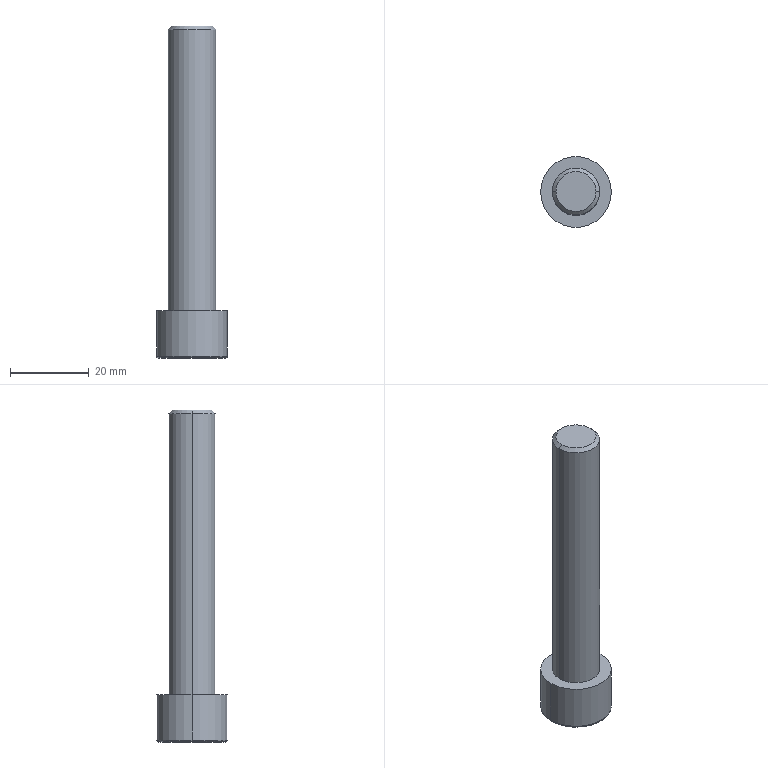Part | Creo | 1 solid | 20 faces | box 18 x 18 x 84.5 mm | volume 10550 mm3 | plane 10 | torus 4 | cylinder 4 | cone 2 | commonest cylinder face diameters 12 x2 18 x2
STEP:
#1=CARTESIAN_POINT('',(56.5,-5.,-119.5));
#2=VERTEX_POINT('',#1);
#3=CARTESIAN_POINT('',(73.5,-5.,-119.5));
#4=VERTEX_POINT('',#3);
#5=CARTESIAN_POINT('',(65.,-5.,-119.5));
#6=DIRECTION('',(0.,0.,-1.));
#7=DIRECTION('',(-1.,0.,0.));
#8=AXIS2_PLACEMENT_3D('',#5,#6,#7);
#9=CIRCLE('',#8,8.5);
#10=EDGE_CURVE('',#2,#4,#9,.T.);
#11=ORIENTED_EDGE('',*,*,#10,.F.);
#12=CARTESIAN_POINT('',(65.,-5.,-119.5));
#13=DIRECTION('',(0.,0.,-1.));
#14=DIRECTION('',(1.,0.,0.));
#15=AXIS2_PLACEMENT_3D('',#12,#13,#14);
#16=CIRCLE('',#15,8.5);
#17=EDGE_CURVE('',#4,#2,#16,.T.);
#18=ORIENTED_EDGE('',*,*,#17,.F.);
#19=EDGE_LOOP('',(#11,#18));
#20=FACE_OUTER_BOUND('',#19,.F.);
#21=CARTESIAN_POINT('',(62.113,0.,-119.5));
#22=VERTEX_POINT('',#21);
#23=CARTESIAN_POINT('',(67.887,0.,-119.5));
#24=VERTEX_POINT('',#23);
#25=CARTESIAN_POINT('',(62.113,0.,-119.5));
#26=DIRECTION('',(1.,0.,0.));
#27=VECTOR('',#26,5.774);
#28=LINE('',#25,#27);
#29=EDGE_CURVE('',#22,#24,#28,.T.);
#30=ORIENTED_EDGE('',*,*,#29,.T.);
#31=CARTESIAN_POINT('',(70.774,-5.,-119.5));
#32=VERTEX_POINT('',#31);
#33=CARTESIAN_POINT('',(70.774,-5.,-119.5));
#34=DIRECTION('',(-0.5,0.866,0.));
#35=VECTOR('',#34,5.774);
#36=LINE('',#33,#35);
#37=EDGE_CURVE('',#32,#24,#36,.T.);
#38=ORIENTED_EDGE('',*,*,#37,.F.);
#39=CARTESIAN_POINT('',(67.887,-10.,-119.5));
#40=VERTEX_POINT('',#39);
#41=CARTESIAN_POINT('',(67.887,-10.,-119.5));
#42=DIRECTION('',(0.5,0.866,0.));
#43=VECTOR('',#42,5.774);
#44=LINE('',#41,#43);
#45=EDGE_CURVE('',#40,#32,#44,.T.);
#46=ORIENTED_EDGE('',*,*,#45,.F.);
#47=CARTESIAN_POINT('',(62.113,-10.,-119.5));
#48=VERTEX_POINT('',#47);
#49=CARTESIAN_POINT('',(67.887,-10.,-119.5));
#50=DIRECTION('',(-1.,0.,0.));
#51=VECTOR('',#50,5.774);
#52=LINE('',#49,#51);
#53=EDGE_CURVE('',#40,#48,#52,.T.);
#54=ORIENTED_EDGE('',*,*,#53,.T.);
#55=CARTESIAN_POINT('',(59.226,-5.,-119.5));
#56=VERTEX_POINT('',#55);
#57=CARTESIAN_POINT('',(59.226,-5.,-119.5));
#58=DIRECTION('',(0.5,-0.866,0.));
#59=VECTOR('',#58,5.774);
#60=LINE('',#57,#59);
#61=EDGE_CURVE('',#56,#48,#60,.T.);
#62=ORIENTED_EDGE('',*,*,#61,.F.);
#63=CARTESIAN_POINT('',(62.113,0.,-119.5));
#64=DIRECTION('',(-0.5,-0.866,0.));
#65=VECTOR('',#64,5.774);
#66=LINE('',#63,#65);
#67=EDGE_CURVE('',#22,#56,#66,.T.);
#68=ORIENTED_EDGE('',*,*,#67,.F.);
#69=EDGE_LOOP('',(#30,#38,#46,#54,#62,#68));
#70=FACE_BOUND('',#69,.F.);
#71=CARTESIAN_POINT('',(65.,-5.,-119.5));
#72=DIRECTION('',(0.,0.,-1.));
#73=DIRECTION('',(-1.,0.,0.));
#74=AXIS2_PLACEMENT_3D('',#71,#72,#73);
#75=PLANE('',#74);
#76=ADVANCED_FACE('',(#20,#70),#75,.T.);
#77=ORIENTED_EDGE('',*,*,#10,.T.);
#78=CARTESIAN_POINT('',(73.854,-5.,-119.354));
#79=VERTEX_POINT('',#78);
#80=CARTESIAN_POINT('',(73.5,-5.,-119.));
#81=DIRECTION('',(0.,1.,0.));
#82=DIRECTION('',(0.7071,0.,-0.7071));
#83=AXIS2_PLACEMENT_3D('',#80,#81,#82);
#84=CIRCLE('',#83,0.5);
#85=EDGE_CURVE('',#79,#4,#84,.T.);
#86=ORIENTED_EDGE('',*,*,#85,.F.);
#87=CARTESIAN_POINT('',(56.146,-5.,-119.354));
#88=VERTEX_POINT('',#87);
#89=CARTESIAN_POINT('',(65.,-5.,-119.354));
#90=DIRECTION('',(0.,0.,-1.));
#91=DIRECTION('',(-1.,0.,0.));
#92=AXIS2_PLACEMENT_3D('',#89,#90,#91);
#93=CIRCLE('',#92,8.854);
#94=EDGE_CURVE('',#88,#79,#93,.T.);
#95=ORIENTED_EDGE('',*,*,#94,.F.);
#96=CARTESIAN_POINT('',(56.5,-5.,-119.));
#97=DIRECTION('',(0.,-1.,0.));
#98=DIRECTION('',(-0.7071,0.,-0.7071));
#99=AXIS2_PLACEMENT_3D('',#96,#97,#98);
#100=CIRCLE('',#99,0.5);
#101=EDGE_CURVE('',#88,#2,#100,.T.);
#102=ORIENTED_EDGE('',*,*,#101,.T.);
#103=EDGE_LOOP('',(#77,#86,#95,#102));
#104=FACE_OUTER_BOUND('',#103,.F.);
#105=CARTESIAN_POINT('',(65.,-5.,-119.));
#106=DIRECTION('',(0.,0.,-1.));
#107=DIRECTION('',(-1.,0.,0.));
#108=AXIS2_PLACEMENT_3D('',#105,#106,#107);
#109=TOROIDAL_SURFACE('',#108,8.5,0.5);
#110=ADVANCED_FACE('',(#104),#109,.T.);
#111=ORIENTED_EDGE('',*,*,#17,.T.);
#112=ORIENTED_EDGE('',*,*,#101,.F.);
#113=CARTESIAN_POINT('',(65.,-5.,-119.354));
#114=DIRECTION('',(0.,0.,-1.));
#115=DIRECTION('',(1.,0.,0.));
#116=AXIS2_PLACEMENT_3D('',#113,#114,#115);
#117=CIRCLE('',#116,8.854);
#118=EDGE_CURVE('',#79,#88,#117,.T.);
#119=ORIENTED_EDGE('',*,*,#118,.F.);
#120=ORIENTED_EDGE('',*,*,#85,.T.);
#121=EDGE_LOOP('',(#111,#112,#119,#120));
#122=FACE_OUTER_BOUND('',#121,.F.);
#123=CARTESIAN_POINT('',(65.,-5.,-119.));
#124=DIRECTION('',(0.,0.,-1.));
#125=DIRECTION('',(-1.,0.,0.));
#126=AXIS2_PLACEMENT_3D('',#123,#124,#125);
#127=TOROIDAL_SURFACE('',#126,8.5,0.5);
#128=ADVANCED_FACE('',(#122),#127,.T.);
#129=CARTESIAN_POINT('',(74.,-5.,-119.));
#130=VERTEX_POINT('',#129);
#131=CARTESIAN_POINT('',(56.,-5.,-119.));
#132=VERTEX_POINT('',#131);
#133=CARTESIAN_POINT('',(65.,-5.,-119.));
#134=DIRECTION('',(0.,0.,-1.));
#135=DIRECTION('',(1.,0.,0.));
#136=AXIS2_PLACEMENT_3D('',#133,#134,#135);
#137=CIRCLE('',#136,9.);
#138=EDGE_CURVE('',#130,#132,#137,.T.);
#139=ORIENTED_EDGE('',*,*,#138,.F.);
#140=CARTESIAN_POINT('',(73.5,-5.,-119.));
#141=DIRECTION('',(0.,1.,0.));
#142=DIRECTION('',(1.,0.,0.));
#143=AXIS2_PLACEMENT_3D('',#140,#141,#142);
#144=CIRCLE('',#143,0.5);
#145=EDGE_CURVE('',#130,#79,#144,.T.);
#146=ORIENTED_EDGE('',*,*,#145,.T.);
#147=ORIENTED_EDGE('',*,*,#118,.T.);
#148=CARTESIAN_POINT('',(56.5,-5.,-119.));
#149=DIRECTION('',(0.,-1.,0.));
#150=DIRECTION('',(-1.,0.,0.));
#151=AXIS2_PLACEMENT_3D('',#148,#149,#150);
#152=CIRCLE('',#151,0.5);
#153=EDGE_CURVE('',#132,#88,#152,.T.);
#154=ORIENTED_EDGE('',*,*,#153,.F.);
#155=EDGE_LOOP('',(#139,#146,#147,#154));
#156=FACE_OUTER_BOUND('',#155,.F.);
#157=CARTESIAN_POINT('',(65.,-5.,-119.));
#158=DIRECTION('',(0.,0.,-1.));
#159=DIRECTION('',(-1.,0.,0.));
#160=AXIS2_PLACEMENT_3D('',#157,#158,#159);
#161=TOROIDAL_SURFACE('',#160,8.5,0.5);
#162=ADVANCED_FACE('',(#156),#161,.T.);
#163=ORIENTED_EDGE('',*,*,#138,.T.);
#164=CARTESIAN_POINT('',(56.,-5.,-107.5));
#165=VERTEX_POINT('',#164);
#166=CARTESIAN_POINT('',(56.,-5.,-107.5));
#167=DIRECTION('',(0.,0.,-1.));
#168=VECTOR('',#167,11.5);
#169=LINE('',#166,#168);
#170=EDGE_CURVE('',#165,#132,#169,.T.);
#171=ORIENTED_EDGE('',*,*,#170,.F.);
#172=CARTESIAN_POINT('',(74.,-5.,-107.5));
#173=VERTEX_POINT('',#172);
#174=CARTESIAN_POINT('',(65.,-5.,-107.5));
#175=DIRECTION('',(0.,0.,1.));
#176=DIRECTION('',(-1.,0.,0.));
#177=AXIS2_PLACEMENT_3D('',#174,#175,#176);
#178=CIRCLE('',#177,9.);
#179=EDGE_CURVE('',#165,#173,#178,.T.);
#180=ORIENTED_EDGE('',*,*,#179,.T.);
#181=CARTESIAN_POINT('',(74.,-5.,-107.5));
#182=DIRECTION('',(0.,0.,-1.));
#183=VECTOR('',#182,11.5);
#184=LINE('',#181,#183);
#185=EDGE_CURVE('',#173,#130,#184,.T.);
#186=ORIENTED_EDGE('',*,*,#185,.T.);
#187=EDGE_LOOP('',(#163,#171,#180,#186));
#188=FACE_OUTER_BOUND('',#187,.F.);
#189=CARTESIAN_POINT('',(65.,-5.,-107.5));
#190=DIRECTION('',(0.,0.,-1.));
#191=DIRECTION('',(-1.,0.,0.));
#192=AXIS2_PLACEMENT_3D('',#189,#190,#191);
#193=CYLINDRICAL_SURFACE('',#192,9.);
#194=ADVANCED_FACE('',(#188),#193,.T.);
#195=CARTESIAN_POINT('',(65.,-5.,-119.));
#196=DIRECTION('',(0.,0.,-1.));
#197=DIRECTION('',(-1.,0.,0.));
#198=AXIS2_PLACEMENT_3D('',#195,#196,#197);
#199=CIRCLE('',#198,9.);
#200=EDGE_CURVE('',#132,#130,#199,.T.);
#201=ORIENTED_EDGE('',*,*,#200,.T.);
#202=ORIENTED_EDGE('',*,*,#185,.F.);
#203=CARTESIAN_POINT('',(65.,-5.,-107.5));
#204=DIRECTION('',(0.,0.,1.));
#205=DIRECTION('',(1.,0.,0.));
#206=AXIS2_PLACEMENT_3D('',#203,#204,#205);
#207=CIRCLE('',#206,9.);
#208=EDGE_CURVE('',#173,#165,#207,.T.);
#209=ORIENTED_EDGE('',*,*,#208,.T.);
#210=ORIENTED_EDGE('',*,*,#170,.T.);
#211=EDGE_LOOP('',(#201,#202,#209,#210));
#212=FACE_OUTER_BOUND('',#211,.F.);
#213=CARTESIAN_POINT('',(65.,-5.,-107.5));
#214=DIRECTION('',(0.,0.,-1.));
#215=DIRECTION('',(-1.,0.,0.));
#216=AXIS2_PLACEMENT_3D('',#213,#214,#215);
#217=CYLINDRICAL_SURFACE('',#216,9.);
#218=ADVANCED_FACE('',(#212),#217,.T.);
#219=ORIENTED_EDGE('',*,*,#200,.F.);
#220=ORIENTED_EDGE('',*,*,#153,.T.);
#221=ORIENTED_EDGE('',*,*,#94,.T.);
#222=ORIENTED_EDGE('',*,*,#145,.F.);
#223=EDGE_LOOP('',(#219,#220,#221,#222));
#224=FACE_OUTER_BOUND('',#223,.F.);
#225=CARTESIAN_POINT('',(65.,-5.,-119.));
#226=DIRECTION('',(0.,0.,-1.));
#227=DIRECTION('',(-1.,0.,0.));
#228=AXIS2_PLACEMENT_3D('',#225,#226,#227);
#229=TOROIDAL_SURFACE('',#228,8.5,0.5);
#230=ADVANCED_FACE('',(#224),#229,.T.);
#231=ORIENTED_EDGE('',*,*,#179,.F.);
#232=ORIENTED_EDGE('',*,*,#208,.F.);
#233=EDGE_LOOP('',(#231,#232));
#234=FACE_OUTER_BOUND('',#233,.F.);
#235=CARTESIAN_POINT('',(59.,-5.,-107.5));
#236=VERTEX_POINT('',#235);
#237=CARTESIAN_POINT('',(71.,-5.,-107.5));
#238=VERTEX_POINT('',#237);
#239=CARTESIAN_POINT('',(65.,-5.,-107.5));
#240=DIRECTION('',(0.,0.,-1.));
#241=DIRECTION('',(-1.,0.,0.));
#242=AXIS2_PLACEMENT_3D('',#239,#240,#241);
#243=CIRCLE('',#242,6.);
#244=EDGE_CURVE('',#236,#238,#243,.T.);
#245=ORIENTED_EDGE('',*,*,#244,.F.);
#246=CARTESIAN_POINT('',(65.,-5.,-107.5));
#247=DIRECTION('',(0.,0.,-1.));
#248=DIRECTION('',(1.,0.,0.));
#249=AXIS2_PLACEMENT_3D('',#246,#247,#248);
#250=CIRCLE('',#249,6.);
#251=EDGE_CURVE('',#238,#236,#250,.T.);
#252=ORIENTED_EDGE('',*,*,#251,.F.);
#253=EDGE_LOOP('',(#245,#252));
#254=FACE_BOUND('',#253,.F.);
#255=CARTESIAN_POINT('',(65.,-5.,-107.5));
#256=DIRECTION('',(0.,0.,1.));
#257=DIRECTION('',(1.,0.,0.));
#258=AXIS2_PLACEMENT_3D('',#255,#256,#257);
#259=PLANE('',#258);
#260=ADVANCED_FACE('',(#234,#254),#259,.T.);
#261=CARTESIAN_POINT('',(71.,-5.,-35.9));
#262=VERTEX_POINT('',#261);
#263=CARTESIAN_POINT('',(59.,-5.,-35.9));
#264=VERTEX_POINT('',#263);
#265=CARTESIAN_POINT('',(65.,-5.,-35.9));
#266=DIRECTION('',(0.,0.,1.));
#267=DIRECTION('',(1.,0.,0.));
#268=AXIS2_PLACEMENT_3D('',#265,#266,#267);
#269=CIRCLE('',#268,6.);
#270=EDGE_CURVE('',#262,#264,#269,.T.);
#271=ORIENTED_EDGE('',*,*,#270,.T.);
#272=CARTESIAN_POINT('',(59.,-5.,-35.9));
#273=DIRECTION('',(0.,0.,-1.));
#274=VECTOR('',#273,71.6);
#275=LINE('',#272,#274);
#276=EDGE_CURVE('',#264,#236,#275,.T.);
#277=ORIENTED_EDGE('',*,*,#276,.T.);
#278=ORIENTED_EDGE('',*,*,#244,.T.);
#279=CARTESIAN_POINT('',(71.,-5.,-35.9));
#280=DIRECTION('',(0.,0.,-1.));
#281=VECTOR('',#280,71.6);
#282=LINE('',#279,#281);
#283=EDGE_CURVE('',#262,#238,#282,.T.);
#284=ORIENTED_EDGE('',*,*,#283,.F.);
#285=EDGE_LOOP('',(#271,#277,#278,#284));
#286=FACE_OUTER_BOUND('',#285,.F.);
#287=CARTESIAN_POINT('',(65.,-5.,-37.5));
#288=DIRECTION('',(0.,0.,-1.));
#289=DIRECTION('',(-1.,0.,0.));
#290=AXIS2_PLACEMENT_3D('',#287,#288,#289);
#291=CYLINDRICAL_SURFACE('',#290,6.);
#292=ADVANCED_FACE('',(#286),#291,.T.);
#293=CARTESIAN_POINT('',(70.1,-5.,-35.));
#294=VERTEX_POINT('',#293);
#295=CARTESIAN_POINT('',(59.9,-5.,-35.));
#296=VERTEX_POINT('',#295);
#297=CARTESIAN_POINT('',(65.,-5.,-35.));
#298=DIRECTION('',(0.,0.,1.));
#299=DIRECTION('',(1.,0.,0.));
#300=AXIS2_PLACEMENT_3D('',#297,#298,#299);
#301=CIRCLE('',#300,5.1);
#302=EDGE_CURVE('',#294,#296,#301,.T.);
#303=ORIENTED_EDGE('',*,*,#302,.T.);
#304=CARTESIAN_POINT('',(59.9,-5.,-35.));
#305=DIRECTION('',(-0.7071,0.,-0.7071));
#306=VECTOR('',#305,1.273);
#307=LINE('',#304,#306);
#308=EDGE_CURVE('',#296,#264,#307,.T.);
#309=ORIENTED_EDGE('',*,*,#308,.T.);
#310=ORIENTED_EDGE('',*,*,#270,.F.);
#311=CARTESIAN_POINT('',(70.1,-5.,-35.));
#312=DIRECTION('',(0.7071,0.,-0.7071));
#313=VECTOR('',#312,1.273);
#314=LINE('',#311,#313);
#315=EDGE_CURVE('',#294,#262,#314,.T.);
#316=ORIENTED_EDGE('',*,*,#315,.F.);
#317=EDGE_LOOP('',(#303,#309,#310,#316));
#318=FACE_OUTER_BOUND('',#317,.F.);
#319=CARTESIAN_POINT('',(65.,-5.,-35.45));
#320=DIRECTION('',(0.,0.,-1.));
#321=DIRECTION('',(-1.,0.,0.));
#322=AXIS2_PLACEMENT_3D('',#319,#320,#321);
#323=CONICAL_SURFACE('',#322,5.55,45.);
#324=ADVANCED_FACE('',(#318),#323,.T.);
#325=CARTESIAN_POINT('',(65.,-5.,-35.));
#326=DIRECTION('',(0.,0.,1.));
#327=DIRECTION('',(-1.,0.,0.));
#328=AXIS2_PLACEMENT_3D('',#325,#326,#327);
#329=CIRCLE('',#328,5.1);
#330=EDGE_CURVE('',#296,#294,#329,.T.);
#331=ORIENTED_EDGE('',*,*,#330,.F.);
#332=ORIENTED_EDGE('',*,*,#302,.F.);
#333=EDGE_LOOP('',(#331,#332));
#334=FACE_OUTER_BOUND('',#333,.F.);
#335=CARTESIAN_POINT('',(65.,-5.,-35.));
#336=DIRECTION('',(0.,0.,-1.));
#337=DIRECTION('',(-1.,0.,0.));
#338=AXIS2_PLACEMENT_3D('',#335,#336,#337);
#339=PLANE('',#338);
#340=ADVANCED_FACE('',(#334),#339,.F.);
#341=ORIENTED_EDGE('',*,*,#330,.T.);
#342=ORIENTED_EDGE('',*,*,#315,.T.);
#343=CARTESIAN_POINT('',(65.,-5.,-35.9));
#344=DIRECTION('',(0.,0.,1.));
#345=DIRECTION('',(-1.,0.,0.));
#346=AXIS2_PLACEMENT_3D('',#343,#344,#345);
#347=CIRCLE('',#346,6.);
#348=EDGE_CURVE('',#264,#262,#347,.T.);
#349=ORIENTED_EDGE('',*,*,#348,.F.);
#350=ORIENTED_EDGE('',*,*,#308,.F.);
#351=EDGE_LOOP('',(#341,#342,#349,#350));
#352=FACE_OUTER_BOUND('',#351,.F.);
#353=CARTESIAN_POINT('',(65.,-5.,-35.45));
#354=DIRECTION('',(0.,0.,-1.));
#355=DIRECTION('',(-1.,0.,0.));
#356=AXIS2_PLACEMENT_3D('',#353,#354,#355);
#357=CONICAL_SURFACE('',#356,5.55,45.);
#358=ADVANCED_FACE('',(#352),#357,.T.);
#359=ORIENTED_EDGE('',*,*,#348,.T.);
#360=ORIENTED_EDGE('',*,*,#283,.T.);
#361=ORIENTED_EDGE('',*,*,#251,.T.);
#362=ORIENTED_EDGE('',*,*,#276,.F.);
#363=EDGE_LOOP('',(#359,#360,#361,#362));
#364=FACE_OUTER_BOUND('',#363,.F.);
#365=CARTESIAN_POINT('',(65.,-5.,-37.5));
#366=DIRECTION('',(0.,0.,-1.));
#367=DIRECTION('',(-1.,0.,0.));
#368=AXIS2_PLACEMENT_3D('',#365,#366,#367);
#369=CYLINDRICAL_SURFACE('',#368,6.);
#370=ADVANCED_FACE('',(#364),#369,.T.);
#371=ORIENTED_EDGE('',*,*,#29,.F.);
#372=CARTESIAN_POINT('',(62.113,0.,-111.58));
#373=VERTEX_POINT('',#372);
#374=CARTESIAN_POINT('',(62.113,0.,-119.5));
#375=DIRECTION('',(0.,0.,1.));
#376=VECTOR('',#375,7.92);
#377=LINE('',#374,#376);
#378=EDGE_CURVE('',#22,#373,#377,.T.);
#379=ORIENTED_EDGE('',*,*,#378,.T.);
#380=CARTESIAN_POINT('',(67.887,0.,-111.58));
#381=VERTEX_POINT('',#380);
#382=CARTESIAN_POINT('',(62.113,0.,-111.58));
#383=DIRECTION('',(1.,0.,0.));
#384=VECTOR('',#383,5.774);
#385=LINE('',#382,#384);
#386=EDGE_CURVE('',#373,#381,#385,.T.);
#387=ORIENTED_EDGE('',*,*,#386,.T.);
#388=CARTESIAN_POINT('',(67.887,0.,-119.5));
#389=DIRECTION('',(0.,0.,1.));
#390=VECTOR('',#389,7.92);
#391=LINE('',#388,#390);
#392=EDGE_CURVE('',#24,#381,#391,.T.);
#393=ORIENTED_EDGE('',*,*,#392,.F.);
#394=EDGE_LOOP('',(#371,#379,#387,#393));
#395=FACE_OUTER_BOUND('',#394,.F.);
#396=CARTESIAN_POINT('',(67.887,0.,-111.58));
#397=DIRECTION('',(0.,-1.,0.));
#398=DIRECTION('',(0.,0.,1.));
#399=AXIS2_PLACEMENT_3D('',#396,#397,#398);
#400=PLANE('',#399);
#401=ADVANCED_FACE('',(#395),#400,.T.);
#402=ORIENTED_EDGE('',*,*,#67,.T.);
#403=CARTESIAN_POINT('',(59.226,-5.,-111.58));
#404=VERTEX_POINT('',#403);
#405=CARTESIAN_POINT('',(59.226,-5.,-119.5));
#406=DIRECTION('',(0.,0.,1.));
#407=VECTOR('',#406,7.92);
#408=LINE('',#405,#407);
#409=EDGE_CURVE('',#56,#404,#408,.T.);
#410=ORIENTED_EDGE('',*,*,#409,.T.);
#411=CARTESIAN_POINT('',(59.226,-5.,-111.58));
#412=DIRECTION('',(0.5,0.866,0.));
#413=VECTOR('',#412,5.774);
#414=LINE('',#411,#413);
#415=EDGE_CURVE('',#404,#373,#414,.T.);
#416=ORIENTED_EDGE('',*,*,#415,.T.);
#417=ORIENTED_EDGE('',*,*,#378,.F.);
#418=EDGE_LOOP('',(#402,#410,#416,#417));
#419=FACE_OUTER_BOUND('',#418,.F.);
#420=CARTESIAN_POINT('',(62.113,0.,-111.58));
#421=DIRECTION('',(0.866,-0.5,0.));
#422=DIRECTION('',(-0.5,-0.866,0.));
#423=AXIS2_PLACEMENT_3D('',#420,#421,#422);
#424=PLANE('',#423);
#425=ADVANCED_FACE('',(#419),#424,.T.);
#426=ORIENTED_EDGE('',*,*,#61,.T.);
#427=CARTESIAN_POINT('',(62.113,-10.,-111.58));
#428=VERTEX_POINT('',#427);
#429=CARTESIAN_POINT('',(62.113,-10.,-119.5));
#430=DIRECTION('',(0.,0.,1.));
#431=VECTOR('',#430,7.92);
#432=LINE('',#429,#431);
#433=EDGE_CURVE('',#48,#428,#432,.T.);
#434=ORIENTED_EDGE('',*,*,#433,.T.);
#435=CARTESIAN_POINT('',(62.113,-10.,-111.58));
#436=DIRECTION('',(-0.5,0.866,0.));
#437=VECTOR('',#436,5.774);
#438=LINE('',#435,#437);
#439=EDGE_CURVE('',#428,#404,#438,.T.);
#440=ORIENTED_EDGE('',*,*,#439,.T.);
#441=ORIENTED_EDGE('',*,*,#409,.F.);
#442=EDGE_LOOP('',(#426,#434,#440,#441));
#443=FACE_OUTER_BOUND('',#442,.F.);
#444=CARTESIAN_POINT('',(59.226,-5.,-111.58));
#445=DIRECTION('',(0.866,0.5,0.));
#446=DIRECTION('',(0.5,-0.866,0.));
#447=AXIS2_PLACEMENT_3D('',#444,#445,#446);
#448=PLANE('',#447);
#449=ADVANCED_FACE('',(#443),#448,.T.);
#450=ORIENTED_EDGE('',*,*,#53,.F.);
#451=CARTESIAN_POINT('',(67.887,-10.,-111.58));
#452=VERTEX_POINT('',#451);
#453=CARTESIAN_POINT('',(67.887,-10.,-119.5));
#454=DIRECTION('',(0.,0.,1.));
#455=VECTOR('',#454,7.92);
#456=LINE('',#453,#455);
#457=EDGE_CURVE('',#40,#452,#456,.T.);
#458=ORIENTED_EDGE('',*,*,#457,.T.);
#459=CARTESIAN_POINT('',(67.887,-10.,-111.58));
#460=DIRECTION('',(-1.,0.,0.));
#461=VECTOR('',#460,5.774);
#462=LINE('',#459,#461);
#463=EDGE_CURVE('',#452,#428,#462,.T.);
#464=ORIENTED_EDGE('',*,*,#463,.T.);
#465=ORIENTED_EDGE('',*,*,#433,.F.);
#466=EDGE_LOOP('',(#450,#458,#464,#465));
#467=FACE_OUTER_BOUND('',#466,.F.);
#468=CARTESIAN_POINT('',(62.113,-10.,-111.58));
#469=DIRECTION('',(0.,1.,0.));
#470=DIRECTION('',(0.,0.,-1.));
#471=AXIS2_PLACEMENT_3D('',#468,#469,#470);
#472=PLANE('',#471);
#473=ADVANCED_FACE('',(#467),#472,.T.);
#474=ORIENTED_EDGE('',*,*,#45,.T.);
#475=CARTESIAN_POINT('',(70.774,-5.,-111.58));
#476=VERTEX_POINT('',#475);
#477=CARTESIAN_POINT('',(70.774,-5.,-119.5));
#478=DIRECTION('',(0.,0.,1.));
#479=VECTOR('',#478,7.92);
#480=LINE('',#477,#479);
#481=EDGE_CURVE('',#32,#476,#480,.T.);
#482=ORIENTED_EDGE('',*,*,#481,.T.);
#483=CARTESIAN_POINT('',(70.774,-5.,-111.58));
#484=DIRECTION('',(-0.5,-0.866,0.));
#485=VECTOR('',#484,5.774);
#486=LINE('',#483,#485);
#487=EDGE_CURVE('',#476,#452,#486,.T.);
#488=ORIENTED_EDGE('',*,*,#487,.T.);
#489=ORIENTED_EDGE('',*,*,#457,.F.);
#490=EDGE_LOOP('',(#474,#482,#488,#489));
#491=FACE_OUTER_BOUND('',#490,.F.);
#492=CARTESIAN_POINT('',(67.887,-10.,-111.58));
#493=DIRECTION('',(-0.866,0.5,0.));
#494=DIRECTION('',(0.5,0.866,0.));
#495=AXIS2_PLACEMENT_3D('',#492,#493,#494);
#496=PLANE('',#495);
#497=ADVANCED_FACE('',(#491),#496,.T.);
#498=ORIENTED_EDGE('',*,*,#37,.T.);
#499=ORIENTED_EDGE('',*,*,#392,.T.);
#500=CARTESIAN_POINT('',(67.887,0.,-111.58));
#501=DIRECTION('',(0.5,-0.866,0.));
#502=VECTOR('',#501,5.774);
#503=LINE('',#500,#502);
#504=EDGE_CURVE('',#381,#476,#503,.T.);
#505=ORIENTED_EDGE('',*,*,#504,.T.);
#506=ORIENTED_EDGE('',*,*,#481,.F.);
#507=EDGE_LOOP('',(#498,#499,#505,#506));
#508=FACE_OUTER_BOUND('',#507,.F.);
#509=CARTESIAN_POINT('',(70.774,-5.,-111.58));
#510=DIRECTION('',(-0.866,-0.5,0.));
#511=DIRECTION('',(-0.5,0.866,0.));
#512=AXIS2_PLACEMENT_3D('',#509,#510,#511);
#513=PLANE('',#512);
#514=ADVANCED_FACE('',(#508),#513,.T.);
#515=ORIENTED_EDGE('',*,*,#415,.F.);
#516=ORIENTED_EDGE('',*,*,#439,.F.);
#517=ORIENTED_EDGE('',*,*,#463,.F.);
#518=ORIENTED_EDGE('',*,*,#487,.F.);
#519=ORIENTED_EDGE('',*,*,#504,.F.);
#520=ORIENTED_EDGE('',*,*,#386,.F.);
#521=EDGE_LOOP('',(#515,#516,#517,#518,#519,#520));
#522=FACE_OUTER_BOUND('',#521,.F.);
#523=CARTESIAN_POINT('',(56.34,-10.,-111.58));
#524=DIRECTION('',(0.,0.,1.));
#525=DIRECTION('',(1.,0.,0.));
#526=AXIS2_PLACEMENT_3D('',#523,#524,#525);
#527=PLANE('',#526);
#528=ADVANCED_FACE('',(#522),#527,.F.);
#529=CLOSED_SHELL('',(#76,#110,#128,#162,#194,#218,#230,#260,#292,#324,#340,#358,#370,#401,#425,#449,#473,#497,#514,#528));
#530=MANIFOLD_SOLID_BREP('',#529);
#531=(LENGTH_UNIT()NAMED_UNIT(*)SI_UNIT(.MILLI.,.METRE.));
#532=UNCERTAINTY_MEASURE_WITH_UNIT(LENGTH_MEASURE(0.008825),#531,'','');
#533=(NAMED_UNIT(*)PLANE_ANGLE_UNIT()SI_UNIT($,.RADIAN.));
#534=PLANE_ANGLE_MEASURE_WITH_UNIT(PLANE_ANGLE_MEASURE(0.01745),#533);
#535=(CONVERSION_BASED_UNIT('DEGREE',#534)NAMED_UNIT(*)PLANE_ANGLE_UNIT());
#536=(NAMED_UNIT(*)SI_UNIT($,.STERADIAN.)SOLID_ANGLE_UNIT());
#537=(GEOMETRIC_REPRESENTATION_CONTEXT(3)GLOBAL_UNCERTAINTY_ASSIGNED_CONTEXT((#532))GLOBAL_UNIT_ASSIGNED_CONTEXT((#531,#535,#536))REPRESENTATION_CONTEXT('',''));
#538=ADVANCED_BREP_SHAPE_REPRESENTATION('',(#530),#537);